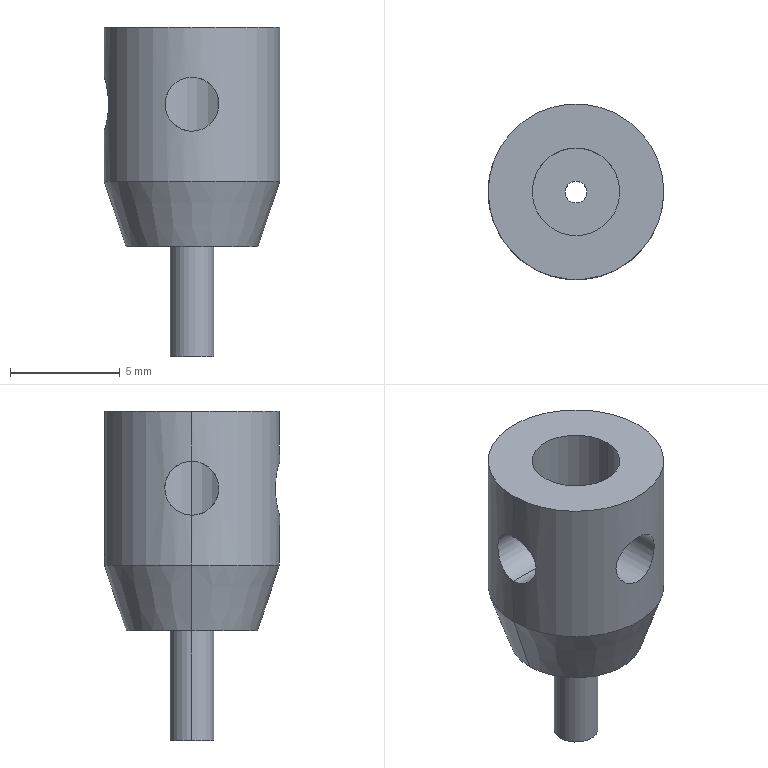Part | SolidWorks | features BaseBody 1 | 1 solid | 18 faces | box 8 x 8 x 15 mm | volume 358.289 mm3 | cylinder 12 | plane 4 | cone 2 | commonest cylinder face diameters 2.459 x4 1 x2 2 x2 4 x2 8 x2
STEP:
#1=CARTESIAN_POINT('',(4.,0.,8.));
#2=VERTEX_POINT('',#1);
#3=CARTESIAN_POINT('',(-4.,0.,8.));
#4=VERTEX_POINT('',#3);
#5=CARTESIAN_POINT('',(0.,0.,8.));
#6=DIRECTION('',(0.,0.,1.));
#7=DIRECTION('',(1.,0.,0.));
#8=AXIS2_PLACEMENT_3D('',#5,#6,#7);
#9=CIRCLE('',#8,4.);
#10=EDGE_CURVE('',#2,#4,#9,.T.);
#11=ORIENTED_EDGE('',*,*,#10,.T.);
#12=CARTESIAN_POINT('',(-4.,0.,10.271));
#13=VERTEX_POINT('',#12);
#14=CARTESIAN_POINT('',(-4.,0.,5.));
#15=DIRECTION('',(0.,0.,1.));
#16=VECTOR('',#15,1000.);
#17=LINE('',#14,#16);
#18=EDGE_CURVE('',#4,#13,#17,.T.);
#19=ORIENTED_EDGE('',*,*,#18,.T.);
#20=CARTESIAN_POINT('',(-4.,0.,12.729));
#21=VERTEX_POINT('',#20);
#22=CARTESIAN_POINT('',(-4.,0.,10.271));
#23=CARTESIAN_POINT('',(-4.,0.1635,10.27));
#24=CARTESIAN_POINT('',(-3.99,0.3238,10.303));
#25=CARTESIAN_POINT('',(-3.954,0.6211,10.427));
#26=CARTESIAN_POINT('',(-3.929,0.7569,10.518));
#27=CARTESIAN_POINT('',(-3.879,0.9821,10.743));
#28=CARTESIAN_POINT('',(-3.854,1.073,10.88));
#29=CARTESIAN_POINT('',(-3.817,1.196,11.175));
#30=CARTESIAN_POINT('',(-3.806,1.229,11.337));
#31=CARTESIAN_POINT('',(-3.806,1.23,11.579));
#32=CARTESIAN_POINT('',(-3.809,1.222,11.661));
#33=CARTESIAN_POINT('',(-3.819,1.19,11.82));
#34=CARTESIAN_POINT('',(-3.826,1.167,11.896));
#35=CARTESIAN_POINT('',(-3.854,1.074,12.121));
#36=CARTESIAN_POINT('',(-3.879,0.9831,12.256));
#37=CARTESIAN_POINT('',(-3.917,0.8132,12.426));
#38=CARTESIAN_POINT('',(-3.929,0.7517,12.476));
#39=CARTESIAN_POINT('',(-3.952,0.6189,12.565));
#40=CARTESIAN_POINT('',(-3.963,0.547,12.604));
#41=CARTESIAN_POINT('',(-3.99,0.3249,12.697));
#42=CARTESIAN_POINT('',(-4.,0.1635,12.729));
#43=CARTESIAN_POINT('',(-4.,0.,12.729));
#44=B_SPLINE_CURVE_WITH_KNOTS('',3,(#22,#23,#24,#25,#26,#27,#28,#29,#30,#31,#32,#33,#34,#35,#36,#37,#38,#39,#40,#41,#42,#43),.UNSPECIFIED.,.F.,.F.,(4,2,2,2,2,2,2,2,2,2,4),(0.003866,0.004349,0.004833,0.005316,0.005799,0.006041,0.006282,0.006766,0.007007,0.007249,0.007732),.UNSPECIFIED.);
#45=EDGE_CURVE('',#13,#21,#44,.T.);
#46=ORIENTED_EDGE('',*,*,#45,.T.);
#47=CARTESIAN_POINT('',(-4.,0.,15.));
#48=VERTEX_POINT('',#47);
#49=CARTESIAN_POINT('',(-4.,0.,5.));
#50=DIRECTION('',(0.,0.,1.));
#51=VECTOR('',#50,1000.);
#52=LINE('',#49,#51);
#53=EDGE_CURVE('',#21,#48,#52,.T.);
#54=ORIENTED_EDGE('',*,*,#53,.T.);
#55=CARTESIAN_POINT('',(4.,0.,15.));
#56=VERTEX_POINT('',#55);
#57=CARTESIAN_POINT('',(0.,0.,15.));
#58=DIRECTION('',(0.,0.,-1.));
#59=DIRECTION('',(1.,0.,0.));
#60=AXIS2_PLACEMENT_3D('',#57,#58,#59);
#61=CIRCLE('',#60,4.);
#62=EDGE_CURVE('',#48,#56,#61,.T.);
#63=ORIENTED_EDGE('',*,*,#62,.T.);
#64=CARTESIAN_POINT('',(4.,0.,5.));
#65=DIRECTION('',(0.,0.,1.));
#66=VECTOR('',#65,1000.);
#67=LINE('',#64,#66);
#68=EDGE_CURVE('',#2,#56,#67,.T.);
#69=ORIENTED_EDGE('',*,*,#68,.F.);
#70=EDGE_LOOP('',(#11,#19,#46,#54,#63,#69));
#71=FACE_OUTER_BOUND('',#70,.T.);
#72=CARTESIAN_POINT('',(0.,0.,5.));
#73=DIRECTION('',(0.,0.,1.));
#74=DIRECTION('',(1.,0.,0.));
#75=AXIS2_PLACEMENT_3D('',#72,#73,#74);
#76=CYLINDRICAL_SURFACE('',#75,4.);
#77=ADVANCED_FACE('',(#71),#76,.T.);
#78=CARTESIAN_POINT('',(3.,0.,5.));
#79=VERTEX_POINT('',#78);
#80=CARTESIAN_POINT('',(-3.,0.,5.));
#81=VERTEX_POINT('',#80);
#82=CARTESIAN_POINT('',(0.,0.,5.));
#83=DIRECTION('',(0.,0.,1.));
#84=DIRECTION('',(1.,0.,0.));
#85=AXIS2_PLACEMENT_3D('',#82,#83,#84);
#86=CIRCLE('',#85,3.);
#87=EDGE_CURVE('',#79,#81,#86,.T.);
#88=ORIENTED_EDGE('',*,*,#87,.T.);
#89=CARTESIAN_POINT('',(-4.,0.,8.));
#90=DIRECTION('',(-0.3162,0.,0.9487));
#91=VECTOR('',#90,1000.);
#92=LINE('',#89,#91);
#93=EDGE_CURVE('',#81,#4,#92,.T.);
#94=ORIENTED_EDGE('',*,*,#93,.T.);
#95=ORIENTED_EDGE('',*,*,#10,.F.);
#96=CARTESIAN_POINT('',(4.,0.,8.));
#97=DIRECTION('',(0.3162,0.,0.9487));
#98=VECTOR('',#97,1000.);
#99=LINE('',#96,#98);
#100=EDGE_CURVE('',#79,#2,#99,.T.);
#101=ORIENTED_EDGE('',*,*,#100,.F.);
#102=EDGE_LOOP('',(#88,#94,#95,#101));
#103=FACE_OUTER_BOUND('',#102,.T.);
#104=CARTESIAN_POINT('',(0.,0.,8.));
#105=DIRECTION('',(0.,0.,1.));
#106=DIRECTION('',(1.,0.,0.));
#107=AXIS2_PLACEMENT_3D('',#104,#105,#106);
#108=CONICAL_SURFACE('',#107,4.,0.3218);
#109=ADVANCED_FACE('',(#103),#108,.T.);
#110=CARTESIAN_POINT('',(-4.,0.,12.729));
#111=CARTESIAN_POINT('',(-4.,-0.1635,12.73));
#112=CARTESIAN_POINT('',(-3.99,-0.3238,12.697));
#113=CARTESIAN_POINT('',(-3.954,-0.6211,12.573));
#114=CARTESIAN_POINT('',(-3.929,-0.7569,12.482));
#115=CARTESIAN_POINT('',(-3.879,-0.9821,12.257));
#116=CARTESIAN_POINT('',(-3.854,-1.073,12.12));
#117=CARTESIAN_POINT('',(-3.817,-1.196,11.825));
#118=CARTESIAN_POINT('',(-3.806,-1.229,11.663));
#119=CARTESIAN_POINT('',(-3.806,-1.23,11.421));
#120=CARTESIAN_POINT('',(-3.809,-1.222,11.339));
#121=CARTESIAN_POINT('',(-3.819,-1.19,11.18));
#122=CARTESIAN_POINT('',(-3.826,-1.167,11.104));
#123=CARTESIAN_POINT('',(-3.854,-1.074,10.879));
#124=CARTESIAN_POINT('',(-3.879,-0.9831,10.744));
#125=CARTESIAN_POINT('',(-3.917,-0.8132,10.574));
#126=CARTESIAN_POINT('',(-3.929,-0.7517,10.524));
#127=CARTESIAN_POINT('',(-3.952,-0.6189,10.435));
#128=CARTESIAN_POINT('',(-3.963,-0.547,10.396));
#129=CARTESIAN_POINT('',(-3.99,-0.3249,10.303));
#130=CARTESIAN_POINT('',(-4.,-0.1635,10.27));
#131=CARTESIAN_POINT('',(-4.,0.,10.271));
#132=B_SPLINE_CURVE_WITH_KNOTS('',3,(#110,#111,#112,#113,#114,#115,#116,#117,#118,#119,#120,#121,#122,#123,#124,#125,#126,#127,#128,#129,#130,#131),.UNSPECIFIED.,.F.,.F.,(4,2,2,2,2,2,2,2,2,2,4),(0.,0.0004833,0.0009665,0.00145,0.001933,0.002175,0.002416,0.0029,0.003141,0.003383,0.003866),.UNSPECIFIED.);
#133=EDGE_CURVE('',#21,#13,#132,.T.);
#134=ORIENTED_EDGE('',*,*,#133,.F.);
#135=CARTESIAN_POINT('',(-2.,0.,12.729));
#136=VERTEX_POINT('',#135);
#137=CARTESIAN_POINT('',(-2.,0.,12.729));
#138=DIRECTION('',(1.,0.,0.));
#139=VECTOR('',#138,1000.);
#140=LINE('',#137,#139);
#141=EDGE_CURVE('',#21,#136,#140,.T.);
#142=ORIENTED_EDGE('',*,*,#141,.T.);
#143=CARTESIAN_POINT('',(-2.,0.,10.271));
#144=VERTEX_POINT('',#143);
#145=CARTESIAN_POINT('',(-2.,0.,10.271));
#146=CARTESIAN_POINT('',(-2.,-0.1661,10.27));
#147=CARTESIAN_POINT('',(-1.978,-0.3311,10.305));
#148=CARTESIAN_POINT('',(-1.905,-0.6283,10.431));
#149=CARTESIAN_POINT('',(-1.853,-0.7613,10.522));
#150=CARTESIAN_POINT('',(-1.747,-0.9816,10.743));
#151=CARTESIAN_POINT('',(-1.691,-1.071,10.875));
#152=CARTESIAN_POINT('',(-1.606,-1.195,11.168));
#153=CARTESIAN_POINT('',(-1.577,-1.229,11.333));
#154=CARTESIAN_POINT('',(-1.577,-1.23,11.667));
#155=CARTESIAN_POINT('',(-1.605,-1.195,11.83));
#156=CARTESIAN_POINT('',(-1.691,-1.071,12.125));
#157=CARTESIAN_POINT('',(-1.747,-0.9815,12.257));
#158=CARTESIAN_POINT('',(-1.854,-0.7596,12.479));
#159=CARTESIAN_POINT('',(-1.905,-0.6285,12.569));
#160=CARTESIAN_POINT('',(-1.979,-0.3294,12.696));
#161=CARTESIAN_POINT('',(-2.,-0.1666,12.73));
#162=CARTESIAN_POINT('',(-2.,0.,12.729));
#163=B_SPLINE_CURVE_WITH_KNOTS('',3,(#145,#146,#147,#148,#149,#150,#151,#152,#153,#154,#155,#156,#157,#158,#159,#160,#161,#162),.UNSPECIFIED.,.F.,.F.,(4,2,2,2,2,2,2,2,4),(0.001977,0.00247,0.002963,0.003455,0.003948,0.004441,0.004934,0.005427,0.00592),.UNSPECIFIED.);
#164=EDGE_CURVE('',#144,#136,#163,.T.);
#165=ORIENTED_EDGE('',*,*,#164,.F.);
#166=CARTESIAN_POINT('',(-2.,0.,10.271));
#167=DIRECTION('',(1.,0.,0.));
#168=VECTOR('',#167,1000.);
#169=LINE('',#166,#168);
#170=EDGE_CURVE('',#13,#144,#169,.T.);
#171=ORIENTED_EDGE('',*,*,#170,.F.);
#172=EDGE_LOOP('',(#134,#142,#165,#171));
#173=FACE_OUTER_BOUND('',#172,.T.);
#174=CARTESIAN_POINT('',(-2.,0.,11.5));
#175=DIRECTION('',(1.,0.,0.));
#176=DIRECTION('',(0.,0.,-1.));
#177=AXIS2_PLACEMENT_3D('',#174,#175,#176);
#178=CYLINDRICAL_SURFACE('',#177,1.229);
#179=ADVANCED_FACE('',(#173),#178,.F.);
#180=CARTESIAN_POINT('',(1.229,-3.806,11.5));
#181=VERTEX_POINT('',#180);
#182=CARTESIAN_POINT('',(-1.23,-3.806,11.5));
#183=VERTEX_POINT('',#182);
#184=CARTESIAN_POINT('',(1.229,-3.806,11.5));
#185=CARTESIAN_POINT('',(1.229,-3.806,11.419));
#186=CARTESIAN_POINT('',(1.221,-3.809,11.337));
#187=CARTESIAN_POINT('',(1.19,-3.819,11.179));
#188=CARTESIAN_POINT('',(1.166,-3.826,11.102));
#189=CARTESIAN_POINT('',(1.073,-3.854,10.878));
#190=CARTESIAN_POINT('',(0.9824,-3.879,10.743));
#191=CARTESIAN_POINT('',(0.8123,-3.917,10.574));
#192=CARTESIAN_POINT('',(0.7507,-3.93,10.523));
#193=CARTESIAN_POINT('',(0.6179,-3.953,10.434));
#194=CARTESIAN_POINT('',(0.5459,-3.963,10.395));
#195=CARTESIAN_POINT('',(0.3237,-3.99,10.303));
#196=CARTESIAN_POINT('',(0.1623,-4.,10.27));
#197=CARTESIAN_POINT('',(-0.1647,-4.,10.271));
#198=CARTESIAN_POINT('',(-0.325,-3.99,10.303));
#199=CARTESIAN_POINT('',(-0.6222,-3.954,10.427));
#200=CARTESIAN_POINT('',(-0.7578,-3.929,10.519));
#201=CARTESIAN_POINT('',(-0.9829,-3.879,10.744));
#202=CARTESIAN_POINT('',(-1.074,-3.854,10.881));
#203=CARTESIAN_POINT('',(-1.197,-3.817,11.176));
#204=CARTESIAN_POINT('',(-1.23,-3.806,11.339));
#205=CARTESIAN_POINT('',(-1.23,-3.806,11.5));
#206=B_SPLINE_CURVE_WITH_KNOTS('',3,(#184,#185,#186,#187,#188,#189,#190,#191,#192,#193,#194,#195,#196,#197,#198,#199,#200,#201,#202,#203,#204,#205),.UNSPECIFIED.,.F.,.F.,(4,2,2,2,2,2,2,2,2,2,4),(0.001934,0.002176,0.002418,0.002901,0.003142,0.003384,0.003867,0.004351,0.004834,0.005317,0.0058),.UNSPECIFIED.);
#207=EDGE_CURVE('',#181,#183,#206,.T.);
#208=ORIENTED_EDGE('',*,*,#207,.F.);
#209=CARTESIAN_POINT('',(1.23,-1.577,11.5));
#210=VERTEX_POINT('',#209);
#211=CARTESIAN_POINT('',(1.23,-2.,11.5));
#212=DIRECTION('',(0.,1.,0.));
#213=VECTOR('',#212,1000.);
#214=LINE('',#211,#213);
#215=EDGE_CURVE('',#181,#210,#214,.T.);
#216=ORIENTED_EDGE('',*,*,#215,.T.);
#217=CARTESIAN_POINT('',(-1.23,-1.577,11.5));
#218=VERTEX_POINT('',#217);
#219=CARTESIAN_POINT('',(-1.23,-1.577,11.5));
#220=CARTESIAN_POINT('',(-1.23,-1.577,11.416));
#221=CARTESIAN_POINT('',(-1.221,-1.584,11.335));
#222=CARTESIAN_POINT('',(-1.189,-1.609,11.175));
#223=CARTESIAN_POINT('',(-1.164,-1.627,11.096));
#224=CARTESIAN_POINT('',(-1.071,-1.691,10.875));
#225=CARTESIAN_POINT('',(-0.9815,-1.747,10.743));
#226=CARTESIAN_POINT('',(-0.761,-1.854,10.522));
#227=CARTESIAN_POINT('',(-0.6284,-1.905,10.431));
#228=CARTESIAN_POINT('',(-0.4066,-1.96,10.337));
#229=CARTESIAN_POINT('',(-0.3273,-1.975,10.312));
#230=CARTESIAN_POINT('',(-0.1671,-1.995,10.279));
#231=CARTESIAN_POINT('',(-0.08558,-2.,10.271));
#232=CARTESIAN_POINT('',(0.1637,-2.,10.27));
#233=CARTESIAN_POINT('',(0.3292,-1.979,10.304));
#234=CARTESIAN_POINT('',(0.627,-1.905,10.43));
#235=CARTESIAN_POINT('',(0.7603,-1.854,10.521));
#236=CARTESIAN_POINT('',(0.9811,-1.747,10.743));
#237=CARTESIAN_POINT('',(1.071,-1.691,10.875));
#238=CARTESIAN_POINT('',(1.195,-1.606,11.168));
#239=CARTESIAN_POINT('',(1.23,-1.577,11.333));
#240=CARTESIAN_POINT('',(1.23,-1.577,11.5));
#241=B_SPLINE_CURVE_WITH_KNOTS('',3,(#219,#220,#221,#222,#223,#224,#225,#226,#227,#228,#229,#230,#231,#232,#233,#234,#235,#236,#237,#238,#239,#240),.UNSPECIFIED.,.F.,.F.,(4,2,2,2,2,2,2,2,2,2,4),(0.,0.0002468,0.0004936,0.0009871,0.001481,0.001728,0.001974,0.002468,0.002961,0.003455,0.003949),.UNSPECIFIED.);
#242=EDGE_CURVE('',#218,#210,#241,.T.);
#243=ORIENTED_EDGE('',*,*,#242,.F.);
#244=CARTESIAN_POINT('',(-1.23,-2.,11.5));
#245=DIRECTION('',(0.,1.,0.));
#246=VECTOR('',#245,1000.);
#247=LINE('',#244,#246);
#248=EDGE_CURVE('',#183,#218,#247,.T.);
#249=ORIENTED_EDGE('',*,*,#248,.F.);
#250=EDGE_LOOP('',(#208,#216,#243,#249));
#251=FACE_OUTER_BOUND('',#250,.T.);
#252=CARTESIAN_POINT('',(0.,-2.,11.5));
#253=DIRECTION('',(0.,1.,0.));
#254=DIRECTION('',(-1.,0.,0.));
#255=AXIS2_PLACEMENT_3D('',#252,#253,#254);
#256=CYLINDRICAL_SURFACE('',#255,1.23);
#257=ADVANCED_FACE('',(#251),#256,.F.);
#258=ORIENTED_EDGE('',*,*,#242,.T.);
#259=CARTESIAN_POINT('',(1.23,-1.577,11.5));
#260=CARTESIAN_POINT('',(1.23,-1.577,11.667));
#261=CARTESIAN_POINT('',(1.195,-1.605,11.83));
#262=CARTESIAN_POINT('',(1.071,-1.691,12.125));
#263=CARTESIAN_POINT('',(0.9819,-1.747,12.256));
#264=CARTESIAN_POINT('',(0.7604,-1.854,12.479));
#265=CARTESIAN_POINT('',(0.6296,-1.905,12.568));
#266=CARTESIAN_POINT('',(0.331,-1.978,12.695));
#267=CARTESIAN_POINT('',(0.1685,-2.,12.729));
#268=CARTESIAN_POINT('',(-0.08116,-2.,12.73));
#269=CARTESIAN_POINT('',(-0.163,-1.995,12.721));
#270=CARTESIAN_POINT('',(-0.3241,-1.975,12.689));
#271=CARTESIAN_POINT('',(-0.4033,-1.96,12.664));
#272=CARTESIAN_POINT('',(-0.626,-1.906,12.57));
#273=CARTESIAN_POINT('',(-0.7594,-1.854,12.48));
#274=CARTESIAN_POINT('',(-0.981,-1.747,12.258));
#275=CARTESIAN_POINT('',(-1.07,-1.692,12.127));
#276=CARTESIAN_POINT('',(-1.195,-1.606,11.831));
#277=CARTESIAN_POINT('',(-1.23,-1.577,11.667));
#278=CARTESIAN_POINT('',(-1.23,-1.577,11.5));
#279=B_SPLINE_CURVE_WITH_KNOTS('',3,(#259,#260,#261,#262,#263,#264,#265,#266,#267,#268,#269,#270,#271,#272,#273,#274,#275,#276,#277,#278),.UNSPECIFIED.,.F.,.F.,(4,2,2,2,2,2,2,2,2,4),(0.003949,0.004441,0.004933,0.005426,0.005918,0.006164,0.00641,0.006903,0.007395,0.007887),.UNSPECIFIED.);
#280=EDGE_CURVE('',#210,#218,#279,.T.);
#281=ORIENTED_EDGE('',*,*,#280,.T.);
#282=EDGE_LOOP('',(#258,#281));
#283=FACE_BOUND('',#282,.T.);
#284=CARTESIAN_POINT('',(-2.,0.,7.));
#285=VERTEX_POINT('',#284);
#286=CARTESIAN_POINT('',(2.,0.,7.));
#287=VERTEX_POINT('',#286);
#288=CARTESIAN_POINT('',(0.,0.,7.));
#289=DIRECTION('',(0.,0.,1.));
#290=DIRECTION('',(1.,0.,0.));
#291=AXIS2_PLACEMENT_3D('',#288,#289,#290);
#292=CIRCLE('',#291,2.);
#293=EDGE_CURVE('',#285,#287,#292,.T.);
#294=ORIENTED_EDGE('',*,*,#293,.F.);
#295=CARTESIAN_POINT('',(-2.,0.,11.));
#296=DIRECTION('',(0.,0.,1.));
#297=VECTOR('',#296,1000.);
#298=LINE('',#295,#297);
#299=EDGE_CURVE('',#285,#144,#298,.T.);
#300=ORIENTED_EDGE('',*,*,#299,.T.);
#301=ORIENTED_EDGE('',*,*,#164,.T.);
#302=CARTESIAN_POINT('',(-2.,0.,15.));
#303=VERTEX_POINT('',#302);
#304=CARTESIAN_POINT('',(-2.,0.,11.));
#305=DIRECTION('',(0.,0.,1.));
#306=VECTOR('',#305,1000.);
#307=LINE('',#304,#306);
#308=EDGE_CURVE('',#136,#303,#307,.T.);
#309=ORIENTED_EDGE('',*,*,#308,.T.);
#310=CARTESIAN_POINT('',(2.,0.,15.));
#311=VERTEX_POINT('',#310);
#312=CARTESIAN_POINT('',(0.,0.,15.));
#313=DIRECTION('',(0.,0.,1.));
#314=DIRECTION('',(1.,0.,0.));
#315=AXIS2_PLACEMENT_3D('',#312,#313,#314);
#316=CIRCLE('',#315,2.);
#317=EDGE_CURVE('',#303,#311,#316,.T.);
#318=ORIENTED_EDGE('',*,*,#317,.T.);
#319=CARTESIAN_POINT('',(2.,0.,11.));
#320=DIRECTION('',(0.,0.,1.));
#321=VECTOR('',#320,1000.);
#322=LINE('',#319,#321);
#323=EDGE_CURVE('',#287,#311,#322,.T.);
#324=ORIENTED_EDGE('',*,*,#323,.F.);
#325=EDGE_LOOP('',(#294,#300,#301,#309,#318,#324));
#326=FACE_OUTER_BOUND('',#325,.T.);
#327=CARTESIAN_POINT('',(0.,0.,11.));
#328=DIRECTION('',(0.,0.,1.));
#329=DIRECTION('',(1.,0.,0.));
#330=AXIS2_PLACEMENT_3D('',#327,#328,#329);
#331=CYLINDRICAL_SURFACE('',#330,2.);
#332=ADVANCED_FACE('',(#283,#326),#331,.F.);
#333=CARTESIAN_POINT('',(1.,0.,0.));
#334=VERTEX_POINT('',#333);
#335=CARTESIAN_POINT('',(-1.,0.,0.));
#336=VERTEX_POINT('',#335);
#337=CARTESIAN_POINT('',(0.,0.,0.));
#338=DIRECTION('',(0.,0.,1.));
#339=DIRECTION('',(1.,0.,0.));
#340=AXIS2_PLACEMENT_3D('',#337,#338,#339);
#341=CIRCLE('',#340,1.);
#342=EDGE_CURVE('',#334,#336,#341,.T.);
#343=ORIENTED_EDGE('',*,*,#342,.T.);
#344=CARTESIAN_POINT('',(-1.,0.,5.));
#345=VERTEX_POINT('',#344);
#346=CARTESIAN_POINT('',(-1.,0.,0.));
#347=DIRECTION('',(0.,0.,1.));
#348=VECTOR('',#347,1000.);
#349=LINE('',#346,#348);
#350=EDGE_CURVE('',#336,#345,#349,.T.);
#351=ORIENTED_EDGE('',*,*,#350,.T.);
#352=CARTESIAN_POINT('',(1.,0.,5.));
#353=VERTEX_POINT('',#352);
#354=CARTESIAN_POINT('',(0.,0.,5.));
#355=DIRECTION('',(0.,0.,1.));
#356=DIRECTION('',(1.,0.,0.));
#357=AXIS2_PLACEMENT_3D('',#354,#355,#356);
#358=CIRCLE('',#357,1.);
#359=EDGE_CURVE('',#353,#345,#358,.T.);
#360=ORIENTED_EDGE('',*,*,#359,.F.);
#361=CARTESIAN_POINT('',(1.,0.,0.));
#362=DIRECTION('',(0.,0.,1.));
#363=VECTOR('',#362,1000.);
#364=LINE('',#361,#363);
#365=EDGE_CURVE('',#334,#353,#364,.T.);
#366=ORIENTED_EDGE('',*,*,#365,.F.);
#367=EDGE_LOOP('',(#343,#351,#360,#366));
#368=FACE_OUTER_BOUND('',#367,.T.);
#369=CARTESIAN_POINT('',(0.,0.,0.));
#370=DIRECTION('',(0.,0.,1.));
#371=DIRECTION('',(1.,0.,0.));
#372=AXIS2_PLACEMENT_3D('',#369,#370,#371);
#373=CYLINDRICAL_SURFACE('',#372,1.);
#374=ADVANCED_FACE('',(#368),#373,.T.);
#375=CARTESIAN_POINT('',(-0.5,0.,0.));
#376=VERTEX_POINT('',#375);
#377=CARTESIAN_POINT('',(0.5,0.,0.));
#378=VERTEX_POINT('',#377);
#379=CARTESIAN_POINT('',(0.,0.,0.));
#380=DIRECTION('',(0.,0.,1.));
#381=DIRECTION('',(1.,0.,0.));
#382=AXIS2_PLACEMENT_3D('',#379,#380,#381);
#383=CIRCLE('',#382,0.5);
#384=EDGE_CURVE('',#376,#378,#383,.T.);
#385=ORIENTED_EDGE('',*,*,#384,.F.);
#386=CARTESIAN_POINT('',(-0.5,0.,7.));
#387=VERTEX_POINT('',#386);
#388=CARTESIAN_POINT('',(-0.5,0.,-0.7446));
#389=DIRECTION('',(0.,0.,1.));
#390=VECTOR('',#389,1000.);
#391=LINE('',#388,#390);
#392=EDGE_CURVE('',#376,#387,#391,.T.);
#393=ORIENTED_EDGE('',*,*,#392,.T.);
#394=CARTESIAN_POINT('',(0.5,0.,7.));
#395=VERTEX_POINT('',#394);
#396=CARTESIAN_POINT('',(0.,0.,7.));
#397=DIRECTION('',(0.,0.,-1.));
#398=DIRECTION('',(1.,0.,0.));
#399=AXIS2_PLACEMENT_3D('',#396,#397,#398);
#400=CIRCLE('',#399,0.5);
#401=EDGE_CURVE('',#395,#387,#400,.T.);
#402=ORIENTED_EDGE('',*,*,#401,.F.);
#403=CARTESIAN_POINT('',(0.5,0.,-0.7446));
#404=DIRECTION('',(0.,0.,1.));
#405=VECTOR('',#404,1000.);
#406=LINE('',#403,#405);
#407=EDGE_CURVE('',#378,#395,#406,.T.);
#408=ORIENTED_EDGE('',*,*,#407,.F.);
#409=EDGE_LOOP('',(#385,#393,#402,#408));
#410=FACE_OUTER_BOUND('',#409,.T.);
#411=CARTESIAN_POINT('',(0.,0.,-0.7446));
#412=DIRECTION('',(0.,0.,1.));
#413=DIRECTION('',(1.,0.,0.));
#414=AXIS2_PLACEMENT_3D('',#411,#412,#413);
#415=CYLINDRICAL_SURFACE('',#414,0.5);
#416=ADVANCED_FACE('',(#410),#415,.F.);
#417=ORIENTED_EDGE('',*,*,#18,.F.);
#418=CARTESIAN_POINT('',(0.,0.,8.));
#419=DIRECTION('',(0.,0.,1.));
#420=DIRECTION('',(1.,0.,0.));
#421=AXIS2_PLACEMENT_3D('',#418,#419,#420);
#422=CIRCLE('',#421,4.);
#423=EDGE_CURVE('',#4,#2,#422,.T.);
#424=ORIENTED_EDGE('',*,*,#423,.T.);
#425=ORIENTED_EDGE('',*,*,#68,.T.);
#426=CARTESIAN_POINT('',(0.,0.,15.));
#427=DIRECTION('',(0.,0.,-1.));
#428=DIRECTION('',(1.,0.,0.));
#429=AXIS2_PLACEMENT_3D('',#426,#427,#428);
#430=CIRCLE('',#429,4.);
#431=EDGE_CURVE('',#56,#48,#430,.T.);
#432=ORIENTED_EDGE('',*,*,#431,.T.);
#433=ORIENTED_EDGE('',*,*,#53,.F.);
#434=ORIENTED_EDGE('',*,*,#133,.T.);
#435=EDGE_LOOP('',(#417,#424,#425,#432,#433,#434));
#436=FACE_OUTER_BOUND('',#435,.T.);
#437=CARTESIAN_POINT('',(-1.23,-3.806,11.5));
#438=CARTESIAN_POINT('',(-1.23,-3.806,11.581));
#439=CARTESIAN_POINT('',(-1.221,-3.809,11.663));
#440=CARTESIAN_POINT('',(-1.19,-3.819,11.821));
#441=CARTESIAN_POINT('',(-1.166,-3.826,11.898));
#442=CARTESIAN_POINT('',(-1.073,-3.854,12.122));
#443=CARTESIAN_POINT('',(-0.9823,-3.879,12.257));
#444=CARTESIAN_POINT('',(-0.8122,-3.917,12.427));
#445=CARTESIAN_POINT('',(-0.7506,-3.93,12.477));
#446=CARTESIAN_POINT('',(-0.6178,-3.953,12.566));
#447=CARTESIAN_POINT('',(-0.5458,-3.963,12.605));
#448=CARTESIAN_POINT('',(-0.3236,-3.99,12.697));
#449=CARTESIAN_POINT('',(-0.1621,-4.,12.73));
#450=CARTESIAN_POINT('',(0.1648,-4.,12.729));
#451=CARTESIAN_POINT('',(0.3251,-3.99,12.697));
#452=CARTESIAN_POINT('',(0.6223,-3.954,12.573));
#453=CARTESIAN_POINT('',(0.7579,-3.929,12.481));
#454=CARTESIAN_POINT('',(0.9829,-3.879,12.256));
#455=CARTESIAN_POINT('',(1.074,-3.854,12.119));
#456=CARTESIAN_POINT('',(1.197,-3.817,11.824));
#457=CARTESIAN_POINT('',(1.229,-3.806,11.661));
#458=CARTESIAN_POINT('',(1.229,-3.806,11.5));
#459=B_SPLINE_CURVE_WITH_KNOTS('',3,(#437,#438,#439,#440,#441,#442,#443,#444,#445,#446,#447,#448,#449,#450,#451,#452,#453,#454,#455,#456,#457,#458),.UNSPECIFIED.,.F.,.F.,(4,2,2,2,2,2,2,2,2,2,4),(0.0058,0.006042,0.006284,0.006767,0.007008,0.00725,0.007733,0.008217,0.0087,0.009183,0.009666),.UNSPECIFIED.);
#460=EDGE_CURVE('',#183,#181,#459,.T.);
#461=ORIENTED_EDGE('',*,*,#460,.T.);
#462=ORIENTED_EDGE('',*,*,#207,.T.);
#463=EDGE_LOOP('',(#461,#462));
#464=FACE_BOUND('',#463,.T.);
#465=CARTESIAN_POINT('',(0.,0.,5.));
#466=DIRECTION('',(0.,0.,1.));
#467=DIRECTION('',(1.,0.,0.));
#468=AXIS2_PLACEMENT_3D('',#465,#466,#467);
#469=CYLINDRICAL_SURFACE('',#468,4.);
#470=ADVANCED_FACE('',(#436,#464),#469,.T.);
#471=ORIENTED_EDGE('',*,*,#93,.F.);
#472=CARTESIAN_POINT('',(0.,0.,5.));
#473=DIRECTION('',(0.,0.,1.));
#474=DIRECTION('',(1.,0.,0.));
#475=AXIS2_PLACEMENT_3D('',#472,#473,#474);
#476=CIRCLE('',#475,3.);
#477=EDGE_CURVE('',#81,#79,#476,.T.);
#478=ORIENTED_EDGE('',*,*,#477,.T.);
#479=ORIENTED_EDGE('',*,*,#100,.T.);
#480=ORIENTED_EDGE('',*,*,#423,.F.);
#481=EDGE_LOOP('',(#471,#478,#479,#480));
#482=FACE_OUTER_BOUND('',#481,.T.);
#483=CARTESIAN_POINT('',(0.,0.,8.));
#484=DIRECTION('',(0.,0.,1.));
#485=DIRECTION('',(1.,0.,0.));
#486=AXIS2_PLACEMENT_3D('',#483,#484,#485);
#487=CONICAL_SURFACE('',#486,4.,0.3218);
#488=ADVANCED_FACE('',(#482),#487,.T.);
#489=ORIENTED_EDGE('',*,*,#141,.F.);
#490=ORIENTED_EDGE('',*,*,#45,.F.);
#491=ORIENTED_EDGE('',*,*,#170,.T.);
#492=CARTESIAN_POINT('',(-2.,0.,12.729));
#493=CARTESIAN_POINT('',(-2.,0.1666,12.73));
#494=CARTESIAN_POINT('',(-1.978,0.3314,12.695));
#495=CARTESIAN_POINT('',(-1.905,0.6285,12.569));
#496=CARTESIAN_POINT('',(-1.853,0.7618,12.478));
#497=CARTESIAN_POINT('',(-1.746,0.9831,12.255));
#498=CARTESIAN_POINT('',(-1.69,1.072,12.124));
#499=CARTESIAN_POINT('',(-1.605,1.196,11.827));
#500=CARTESIAN_POINT('',(-1.577,1.23,11.662));
#501=CARTESIAN_POINT('',(-1.578,1.229,11.412));
#502=CARTESIAN_POINT('',(-1.585,1.22,11.33));
#503=CARTESIAN_POINT('',(-1.61,1.187,11.171));
#504=CARTESIAN_POINT('',(-1.628,1.163,11.092));
#505=CARTESIAN_POINT('',(-1.692,1.069,10.872));
#506=CARTESIAN_POINT('',(-1.748,0.9793,10.74));
#507=CARTESIAN_POINT('',(-1.855,0.7584,10.52));
#508=CARTESIAN_POINT('',(-1.906,0.6257,10.43));
#509=CARTESIAN_POINT('',(-1.96,0.4039,10.336));
#510=CARTESIAN_POINT('',(-1.975,0.3245,10.311));
#511=CARTESIAN_POINT('',(-1.995,0.1645,10.279));
#512=CARTESIAN_POINT('',(-2.,0.08304,10.27));
#513=CARTESIAN_POINT('',(-2.,0.,10.271));
#514=B_SPLINE_CURVE_WITH_KNOTS('',3,(#492,#493,#494,#495,#496,#497,#498,#499,#500,#501,#502,#503,#504,#505,#506,#507,#508,#509,#510,#511,#512,#513),.UNSPECIFIED.,.F.,.F.,(4,2,2,2,2,2,2,2,2,2,4),(0.00592,0.006413,0.006906,0.007399,0.007892,0.008138,0.008385,0.008878,0.009371,0.009617,0.009864),.UNSPECIFIED.);
#515=EDGE_CURVE('',#136,#144,#514,.T.);
#516=ORIENTED_EDGE('',*,*,#515,.F.);
#517=EDGE_LOOP('',(#489,#490,#491,#516));
#518=FACE_OUTER_BOUND('',#517,.T.);
#519=CARTESIAN_POINT('',(-2.,0.,11.5));
#520=DIRECTION('',(1.,0.,0.));
#521=DIRECTION('',(0.,0.,-1.));
#522=AXIS2_PLACEMENT_3D('',#519,#520,#521);
#523=CYLINDRICAL_SURFACE('',#522,1.229);
#524=ADVANCED_FACE('',(#518),#523,.F.);
#525=ORIENTED_EDGE('',*,*,#215,.F.);
#526=ORIENTED_EDGE('',*,*,#460,.F.);
#527=ORIENTED_EDGE('',*,*,#248,.T.);
#528=ORIENTED_EDGE('',*,*,#280,.F.);
#529=EDGE_LOOP('',(#525,#526,#527,#528));
#530=FACE_OUTER_BOUND('',#529,.T.);
#531=CARTESIAN_POINT('',(0.,-2.,11.5));
#532=DIRECTION('',(0.,1.,0.));
#533=DIRECTION('',(-1.,0.,0.));
#534=AXIS2_PLACEMENT_3D('',#531,#532,#533);
#535=CYLINDRICAL_SURFACE('',#534,1.23);
#536=ADVANCED_FACE('',(#530),#535,.F.);
#537=CARTESIAN_POINT('',(0.,0.,15.));
#538=DIRECTION('',(0.,0.,1.));
#539=DIRECTION('',(1.,0.,0.));
#540=AXIS2_PLACEMENT_3D('',#537,#538,#539);
#541=CIRCLE('',#540,2.);
#542=EDGE_CURVE('',#311,#303,#541,.T.);
#543=ORIENTED_EDGE('',*,*,#542,.F.);
#544=ORIENTED_EDGE('',*,*,#317,.F.);
#545=EDGE_LOOP('',(#543,#544));
#546=FACE_BOUND('',#545,.T.);
#547=ORIENTED_EDGE('',*,*,#431,.F.);
#548=ORIENTED_EDGE('',*,*,#62,.F.);
#549=EDGE_LOOP('',(#547,#548));
#550=FACE_OUTER_BOUND('',#549,.T.);
#551=CARTESIAN_POINT('',(0.,0.,15.));
#552=DIRECTION('',(0.,0.,-1.));
#553=DIRECTION('',(-1.,0.,0.));
#554=AXIS2_PLACEMENT_3D('',#551,#552,#553);
#555=PLANE('',#554);
#556=ADVANCED_FACE('',(#546,#550),#555,.F.);
#557=ORIENTED_EDGE('',*,*,#359,.T.);
#558=CARTESIAN_POINT('',(0.,0.,5.));
#559=DIRECTION('',(0.,0.,1.));
#560=DIRECTION('',(1.,0.,0.));
#561=AXIS2_PLACEMENT_3D('',#558,#559,#560);
#562=CIRCLE('',#561,1.);
#563=EDGE_CURVE('',#345,#353,#562,.T.);
#564=ORIENTED_EDGE('',*,*,#563,.T.);
#565=EDGE_LOOP('',(#557,#564));
#566=FACE_BOUND('',#565,.T.);
#567=ORIENTED_EDGE('',*,*,#87,.F.);
#568=ORIENTED_EDGE('',*,*,#477,.F.);
#569=EDGE_LOOP('',(#567,#568));
#570=FACE_OUTER_BOUND('',#569,.T.);
#571=CARTESIAN_POINT('',(0.,0.,5.));
#572=DIRECTION('',(0.,0.,-1.));
#573=DIRECTION('',(-1.,0.,0.));
#574=AXIS2_PLACEMENT_3D('',#571,#572,#573);
#575=PLANE('',#574);
#576=ADVANCED_FACE('',(#566,#570),#575,.T.);
#577=ORIENTED_EDGE('',*,*,#299,.F.);
#578=CARTESIAN_POINT('',(0.,0.,7.));
#579=DIRECTION('',(0.,0.,1.));
#580=DIRECTION('',(1.,0.,0.));
#581=AXIS2_PLACEMENT_3D('',#578,#579,#580);
#582=CIRCLE('',#581,2.);
#583=EDGE_CURVE('',#287,#285,#582,.T.);
#584=ORIENTED_EDGE('',*,*,#583,.F.);
#585=ORIENTED_EDGE('',*,*,#323,.T.);
#586=ORIENTED_EDGE('',*,*,#542,.T.);
#587=ORIENTED_EDGE('',*,*,#308,.F.);
#588=ORIENTED_EDGE('',*,*,#515,.T.);
#589=EDGE_LOOP('',(#577,#584,#585,#586,#587,#588));
#590=FACE_OUTER_BOUND('',#589,.T.);
#591=CARTESIAN_POINT('',(0.,0.,11.));
#592=DIRECTION('',(0.,0.,1.));
#593=DIRECTION('',(1.,0.,0.));
#594=AXIS2_PLACEMENT_3D('',#591,#592,#593);
#595=CYLINDRICAL_SURFACE('',#594,2.);
#596=ADVANCED_FACE('',(#590),#595,.F.);
#597=ORIENTED_EDGE('',*,*,#350,.F.);
#598=CARTESIAN_POINT('',(0.,0.,0.));
#599=DIRECTION('',(0.,0.,1.));
#600=DIRECTION('',(1.,0.,0.));
#601=AXIS2_PLACEMENT_3D('',#598,#599,#600);
#602=CIRCLE('',#601,1.);
#603=EDGE_CURVE('',#336,#334,#602,.T.);
#604=ORIENTED_EDGE('',*,*,#603,.T.);
#605=ORIENTED_EDGE('',*,*,#365,.T.);
#606=ORIENTED_EDGE('',*,*,#563,.F.);
#607=EDGE_LOOP('',(#597,#604,#605,#606));
#608=FACE_OUTER_BOUND('',#607,.T.);
#609=CARTESIAN_POINT('',(0.,0.,0.));
#610=DIRECTION('',(0.,0.,1.));
#611=DIRECTION('',(1.,0.,0.));
#612=AXIS2_PLACEMENT_3D('',#609,#610,#611);
#613=CYLINDRICAL_SURFACE('',#612,1.);
#614=ADVANCED_FACE('',(#608),#613,.T.);
#615=ORIENTED_EDGE('',*,*,#401,.T.);
#616=CARTESIAN_POINT('',(0.,0.,7.));
#617=DIRECTION('',(0.,0.,-1.));
#618=DIRECTION('',(1.,0.,0.));
#619=AXIS2_PLACEMENT_3D('',#616,#617,#618);
#620=CIRCLE('',#619,0.5);
#621=EDGE_CURVE('',#387,#395,#620,.T.);
#622=ORIENTED_EDGE('',*,*,#621,.T.);
#623=EDGE_LOOP('',(#615,#622));
#624=FACE_BOUND('',#623,.T.);
#625=ORIENTED_EDGE('',*,*,#583,.T.);
#626=ORIENTED_EDGE('',*,*,#293,.T.);
#627=EDGE_LOOP('',(#625,#626));
#628=FACE_OUTER_BOUND('',#627,.T.);
#629=CARTESIAN_POINT('',(0.,0.,7.));
#630=DIRECTION('',(0.,0.,1.));
#631=DIRECTION('',(1.,0.,0.));
#632=AXIS2_PLACEMENT_3D('',#629,#630,#631);
#633=PLANE('',#632);
#634=ADVANCED_FACE('',(#624,#628),#633,.T.);
#635=CARTESIAN_POINT('',(0.,0.,0.));
#636=DIRECTION('',(0.,0.,1.));
#637=DIRECTION('',(1.,0.,0.));
#638=AXIS2_PLACEMENT_3D('',#635,#636,#637);
#639=CIRCLE('',#638,0.5);
#640=EDGE_CURVE('',#378,#376,#639,.T.);
#641=ORIENTED_EDGE('',*,*,#640,.T.);
#642=ORIENTED_EDGE('',*,*,#384,.T.);
#643=EDGE_LOOP('',(#641,#642));
#644=FACE_BOUND('',#643,.T.);
#645=ORIENTED_EDGE('',*,*,#342,.F.);
#646=ORIENTED_EDGE('',*,*,#603,.F.);
#647=EDGE_LOOP('',(#645,#646));
#648=FACE_OUTER_BOUND('',#647,.T.);
#649=CARTESIAN_POINT('',(0.,0.,0.));
#650=DIRECTION('',(0.,0.,-1.));
#651=DIRECTION('',(-1.,0.,0.));
#652=AXIS2_PLACEMENT_3D('',#649,#650,#651);
#653=PLANE('',#652);
#654=ADVANCED_FACE('',(#644,#648),#653,.T.);
#655=ORIENTED_EDGE('',*,*,#392,.F.);
#656=ORIENTED_EDGE('',*,*,#640,.F.);
#657=ORIENTED_EDGE('',*,*,#407,.T.);
#658=ORIENTED_EDGE('',*,*,#621,.F.);
#659=EDGE_LOOP('',(#655,#656,#657,#658));
#660=FACE_OUTER_BOUND('',#659,.T.);
#661=CARTESIAN_POINT('',(0.,0.,-0.7446));
#662=DIRECTION('',(0.,0.,1.));
#663=DIRECTION('',(1.,0.,0.));
#664=AXIS2_PLACEMENT_3D('',#661,#662,#663);
#665=CYLINDRICAL_SURFACE('',#664,0.5);
#666=ADVANCED_FACE('',(#660),#665,.F.);
#667=CLOSED_SHELL('',(#77,#109,#179,#257,#332,#374,#416,#470,#488,#524,#536,#556,#576,#596,#614,#634,#654,#666));
#668=MANIFOLD_SOLID_BREP('',#667);
#669=CARTESIAN_POINT('',(0.,0.,0.));
#670=DIRECTION('',(0.,0.,1.));
#671=DIRECTION('',(1.,0.,0.));
#672=AXIS2_PLACEMENT_3D('',#669,#670,#671);
#673=(LENGTH_UNIT()NAMED_UNIT(*)SI_UNIT(.MILLI.,.METRE.));
#674=UNCERTAINTY_MEASURE_WITH_UNIT(LENGTH_MEASURE(0.00001),#673,'','');
#675=(NAMED_UNIT(*)PLANE_ANGLE_UNIT()SI_UNIT($,.RADIAN.));
#676=(NAMED_UNIT(*)SI_UNIT($,.STERADIAN.)SOLID_ANGLE_UNIT());
#677=(GEOMETRIC_REPRESENTATION_CONTEXT(3)GLOBAL_UNCERTAINTY_ASSIGNED_CONTEXT((#674))GLOBAL_UNIT_ASSIGNED_CONTEXT((#673,#675,#676))REPRESENTATION_CONTEXT('',''));
#678=ADVANCED_BREP_SHAPE_REPRESENTATION('',(#668,#672),#677);